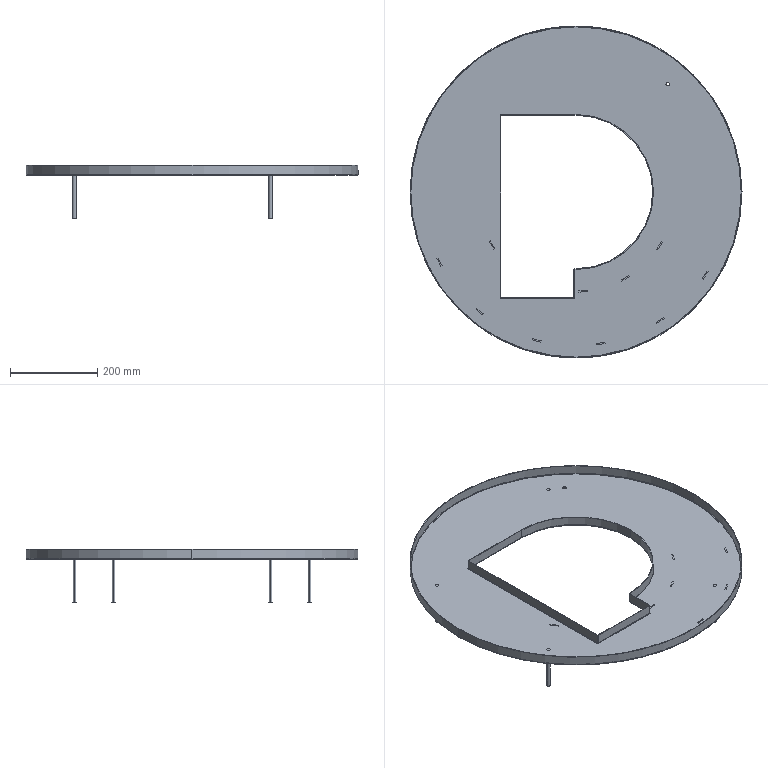Part | 1 solid | 143 faces | box 760 x 760 x 123 mm | volume 516052 mm3 | plane 99 | cylinder 28 | torus 8 | spline 8 | commonest cylinder face diameters 8 x10 1.473 x5 3.873 x5 351.18 x2 353.58 x2 757.6 x2